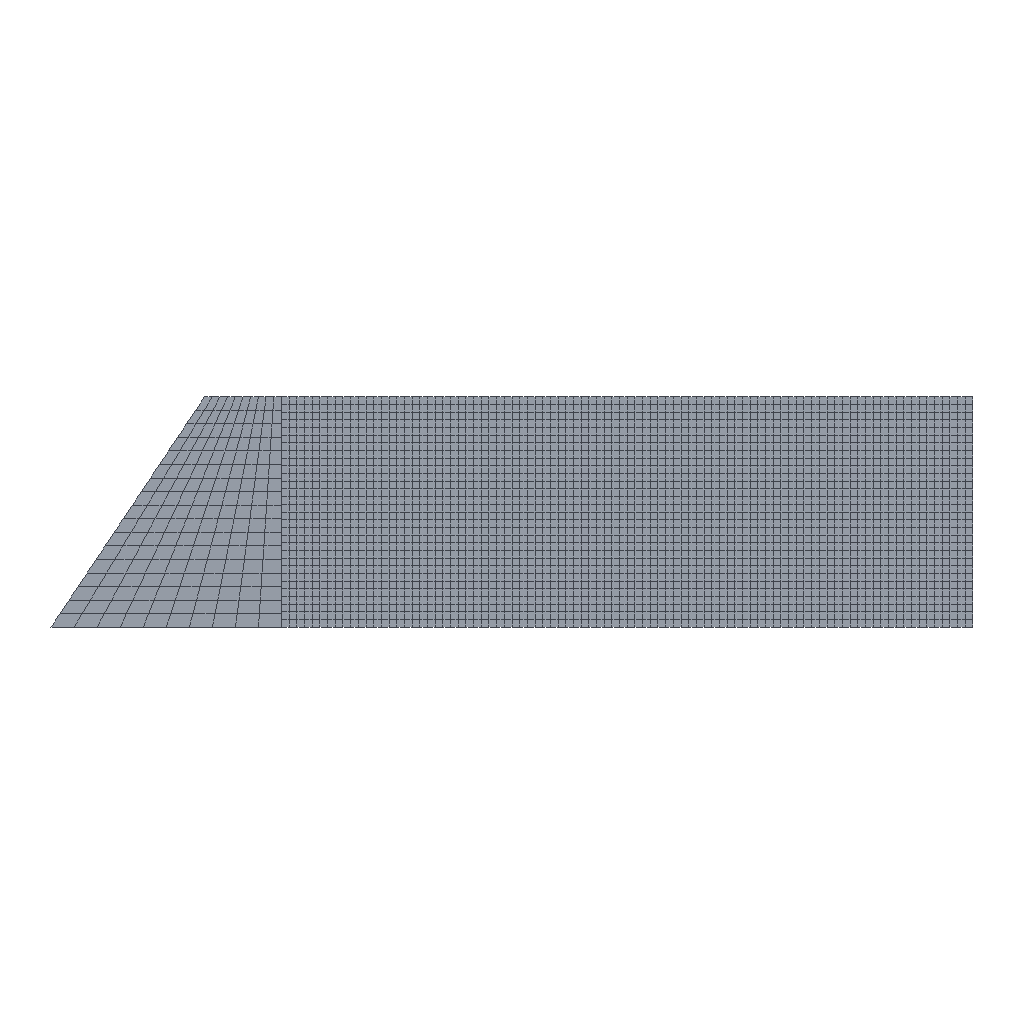Simulation study | abaqus
Set-up summary:
category,name,step,type,value,unit,region
solver,abaqus,,Abaqus/CAE 2024
units,unstated,,unstated,E=50000 density=1.7 (no match)
analysis,load,,static,time_period=1
analysis,move,,static,time_period=1
mesh,nodes,,,3019
mesh,elements,,,2870
element_type,CPE4,,,2870
material,soil,,E,50000
material,soil,,nu,0.3
material,soil,,density,1.7
material,soil,,behaviors,plastic; mohr coulomb; mohr coulomb hardening
material,wall,,E,2e+07
material,wall,,nu,0.2
section,soil,,solid section,,,_PickedSet16
section,wall,,solid section,,,_PickedSet6
load,Load-1,load,gravity,10,,_PickedSet8
load,Load-2,load,pressure,7,,_PickedSurf9
bc,BC-1,initial,fixed,"[dofs=x,y n=2]",,_PickedSet16
bc,BC-2,initial,fixed,[dofs=x],,_PickedSet7
bc,BC-3,load,fixed,"[dofs=x,y n=2]",,_PickedSet23
bc,BC-4,load,fixed,"[dofs=x,y n=2]",,_PickedSet24
bc,BC-1,move,fixed,"[dofs=x,y n=2]",,_PickedSet16
bc,BC-2,move,fixed,[dofs=x],,_PickedSet7
bc,BC-3,move,displacement,0.003 [dofs=y],,_PickedSet23
bc,BC-4,move,fixed,"[dofs=x,y n=2]",,_PickedSet24
contact,Int-1,initial,contact pair surface to surface,interaction=wall-soil; friction=0; behavior=hard,,soil-1.soil-int / wall-1.wall-int
Abaqus input file, long lists of numbers shortened:
*Heading
** Job name: deck Model name: Model-1
** Generated by: Abaqus/CAE 2024
*Preprint, echo=NO, model=NO, history=NO, contact=NO
**
** PARTS
**
*Part, name=soil
*Node
      1,           0.,           0.
      2,  0.1,           0.
** (2819 more lines like these left out)
*Element, type=CPE4
   1,    1,    2,   93,   92
   2,    2,    3,   94,   93
** (2698 more lines like these left out)
*Nset, nset=_PickedSet16, internal, generate
    1,  2821,     1
*Elset, elset=_PickedSet16, internal, generate
    1,  2700,     1
*Elset, elset=_soil-int_S4, internal, generate
    1,  2611,    90
*Surface, type=ELEMENT, name=soil-int
_soil-int_S4, S4
** Section: soil
*Solid Section, elset=_PickedSet16, material=soil
,
*End Part
**
*Part, name=wall
*Node
      1,          -3.,           0.
      2,  -2.7,           0.
** (196 more lines like these left out)
*Element, type=CPE4
  1,   1,   2,  13,  12
  2,   2,   3,  14,  13
** (168 more lines like these left out)
*Nset, nset=_PickedSet6, internal, generate
   1,  198,    1
*Elset, elset=_PickedSet6, internal, generate
   1,  170,    1
*Elset, elset=_wall-int_S2, internal, generate
  10,  170,   10
*Surface, type=ELEMENT, name=wall-int
_wall-int_S2, S2
** Section: wall
*Solid Section, elset=_PickedSet6, material=wall
,
*End Part
**
**
** ASSEMBLY
**
*Assembly, name=Assembly
**
*Instance, name=soil-1, part=soil
*End Instance
**
*Instance, name=wall-1, part=wall
*End Instance
**
*Nset, nset=_PickedSet7, internal, instance=soil-1, generate
   91,  2821,    91
*Elset, elset=_PickedSet7, internal, instance=soil-1, generate
   90,  2700,    90
*Nset, nset=_PickedSet8, internal, instance=soil-1, generate
    1,  2821,     1
*Elset, elset=_PickedSet8, internal, instance=soil-1, generate
    1,  2700,     1
*Nset, nset=_PickedSet16, internal, instance=soil-1, generate
  1,  91,   1
*Elset, elset=_PickedSet16, internal, instance=soil-1, generate
  1,  90,   1
*Nset, nset=_PickedSet23, internal, instance=wall-1
 188,
*Nset, nset=_PickedSet24, internal, instance=wall-1
 11,
*Elset, elset=__PickedSurf9_S3, internal, instance=soil-1, generate
 2611,  2700,     1
*Surface, type=ELEMENT, name=_PickedSurf9, internal
__PickedSurf9_S3, S3
*Nset, nset=_T-New, internal
_PickedSet23,
*Transform, nset=_T-New, type=C
          0.,       -0.001,           0.,           0.,       -0.001,           1.
*End Assembly
**
** MATERIALS
**
*Material, name=soil
*Density
 1.7,
*Elastic
50000., 0.3
*Mohr Coulomb
37.,10.
*Mohr Coulomb Hardening
 0.1,0.
*Material, name=wall
*Elastic
 2e+07, 0.2
**
** INTERACTION PROPERTIES
**
*Surface Interaction, name=wall-soil
1.,
*Friction
0.,
*Surface Behavior, pressure-overclosure=HARD
**
** BOUNDARY CONDITIONS
**
** Name: BC-1 Type: Displacement/Rotation
*Boundary
_PickedSet16, 1, 1
_PickedSet16, 2, 2
** Name: BC-2 Type: Displacement/Rotation
*Boundary
_PickedSet7, 1, 1
**
** INTERACTIONS
**
** Interaction: Int-1
*Contact Pair, interaction=wall-soil, type=SURFACE TO SURFACE
soil-1.soil-int, wall-1.wall-int
** ----------------------------------------------------------------
**
** STEP: load
**
*Step, name=load, nlgeom=NO, unsymm=YES
*Static
0.1, 1., 1e-05, 0.2
**
** BOUNDARY CONDITIONS
**
** Name: BC-3 Type: Displacement/Rotation
*Boundary
_PickedSet23, 1, 1
_PickedSet23, 2, 2
** Name: BC-4 Type: Displacement/Rotation
*Boundary
_PickedSet24, 1, 1
_PickedSet24, 2, 2
**
** LOADS
**
** Name: Load-1   Type: Gravity
*Dload
_PickedSet8, GRAV, 10., 0., -1.
** Name: Load-2   Type: Pressure
*Dsload
_PickedSurf9, P, 7.
**
** OUTPUT REQUESTS
**
*Restart, write, frequency=0
**
** FIELD OUTPUT: F-Output-1
**
*Output, field, variable=PRESELECT
**
** HISTORY OUTPUT: H-Output-1
**
*Output, history, variable=PRESELECT
*End Step
** ----------------------------------------------------------------
**
** STEP: move
**
*Step, name=move, nlgeom=NO, unsymm=YES
*Static
0.1, 1., 1e-05, 0.2
**
** BOUNDARY CONDITIONS
**
** Name: BC-1 Type: Displacement/Rotation
*Boundary, op=NEW
_PickedSet16, 1, 1
_PickedSet16, 2, 2
** Name: BC-2 Type: Displacement/Rotation
*Boundary, op=NEW
_PickedSet7, 1, 1
** Name: BC-3 Type: Displacement/Rotation
*Boundary, op=NEW
_PickedSet23, 2, 2, 0.003
** Name: BC-4 Type: Displacement/Rotation
*Boundary, op=NEW
_PickedSet24, 1, 1
_PickedSet24, 2, 2
**
** OUTPUT REQUESTS
**
*Restart, write, frequency=0
**
** FIELD OUTPUT: F-Output-1
**
*Output, field, variable=PRESELECT
**
** HISTORY OUTPUT: H-Output-1
**
*Output, history, variable=PRESELECT
*End Step
Results summary:
result,odb.job_status,,,JOB_STATUS_COMPLETED_SUCCESSFULLY,"consistent, unstated (Abaqus has no unit system)"
result,steps[0].procedure,load,,*STATIC,"consistent, unstated (Abaqus has no unit system)"
result,steps[0].time_period,load,,1,"consistent, unstated (Abaqus has no unit system)"
result,steps[0].n_frames,load,,8,"consistent, unstated (Abaqus has no unit system)"
result,steps[0].last_frame.id,load,,7,"consistent, unstated (Abaqus has no unit system)"
result,steps[0].last_frame.value,load,,1,"consistent, unstated (Abaqus has no unit system)"
result,steps[0].last_frame.description,load,,Increment      7: Step Time =    1.000,"consistent, unstated (Abaqus has no unit system)"
result,steps[0].completed,load,,True,"consistent, unstated (Abaqus has no unit system)"
result,steps[0].max_U_magnitude,load,,0.001453,"consistent, unstated (Abaqus has no unit system)"
result,steps[0].max_S_mises,load,,248.343,"consistent, unstated (Abaqus has no unit system)"
result,steps[0].RF_sum[1],load,,0,"consistent, unstated (Abaqus has no unit system)"
result,steps[0].RF_sum[2],load,,522,"consistent, unstated (Abaqus has no unit system)"
result,steps[1].procedure,move,,*STATIC,"consistent, unstated (Abaqus has no unit system)"
result,steps[1].time_period,move,,1,"consistent, unstated (Abaqus has no unit system)"
result,steps[1].n_frames,move,,8,"consistent, unstated (Abaqus has no unit system)"
result,steps[1].last_frame.id,move,,7,"consistent, unstated (Abaqus has no unit system)"
result,steps[1].last_frame.value,move,,1,"consistent, unstated (Abaqus has no unit system)"
result,steps[1].last_frame.description,move,,Increment      7: Step Time =    1.000,"consistent, unstated (Abaqus has no unit system)"
result,steps[1].completed,move,,True,"consistent, unstated (Abaqus has no unit system)"
result,steps[1].max_U_magnitude,move,,0.004643,"consistent, unstated (Abaqus has no unit system)"
result,steps[1].max_S_mises,move,,143.252,"consistent, unstated (Abaqus has no unit system)"
result,steps[1].RF_sum[1],move,,2.86102e-06,"consistent, unstated (Abaqus has no unit system)"
result,steps[1].RF_sum[2],move,,522,"consistent, unstated (Abaqus has no unit system)"